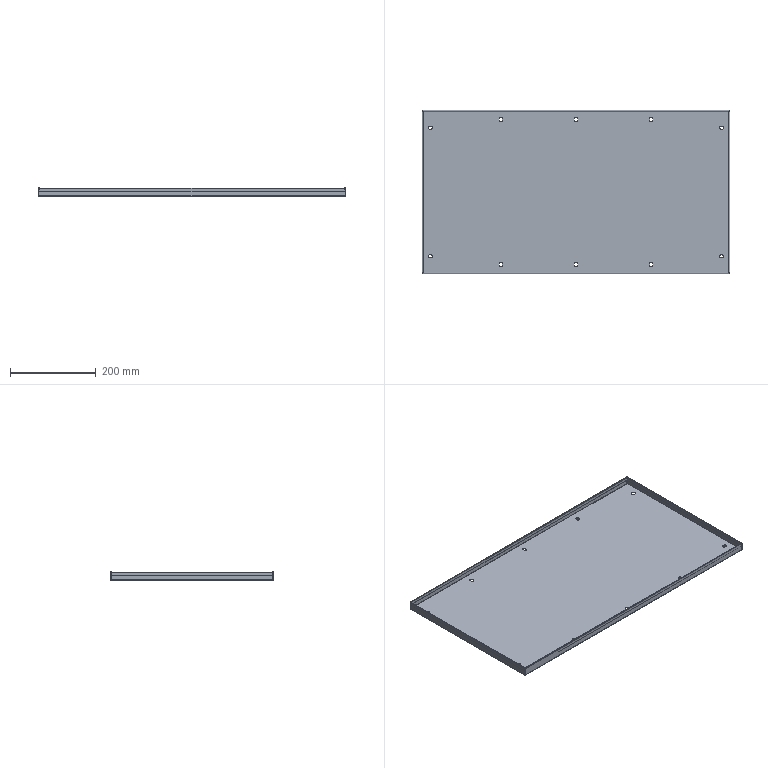Part | STEP file | Magazine plate | 1 solid | 114 faces | box 717 x 380 x 20 mm | volume 394457 mm3 | plane 66 | cylinder 40 | spline 8 | commonest cylinder face diameters 7 x24 0.1 x4 0.2 x4 2.5 x4 2.6 x4